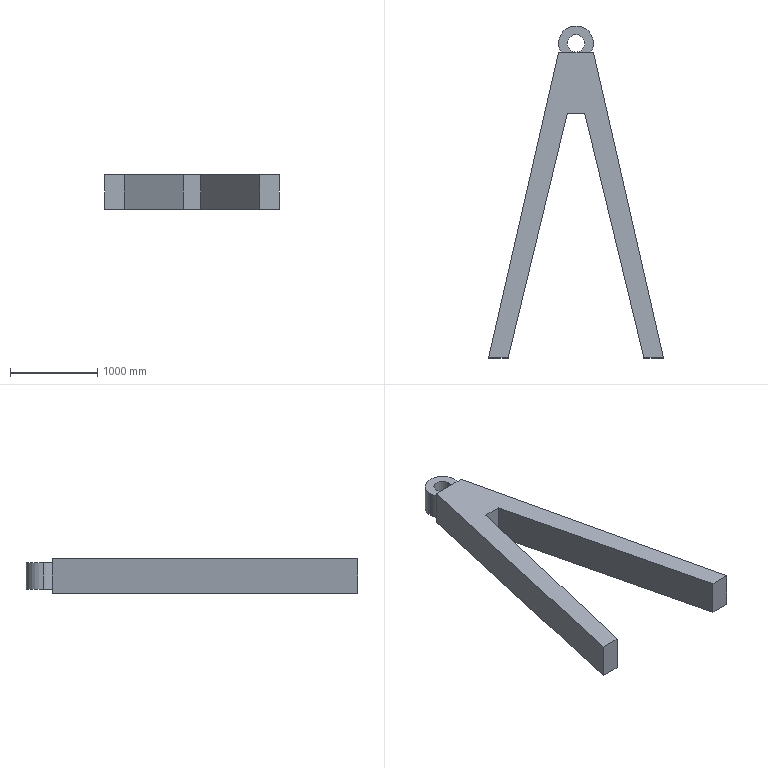Part | SolidWorks | features ICE 2, Extrusion 1 | 1 solid | 17 faces | box 2000 x 3800 x 400 mm | volume 719938598 mm3 | plane 12 | cylinder 5 | commonest cylinder face diameters 400 x3 200 x2
STEP:
#1=CARTESIAN_POINT('',(-100.,0.,-150.));
#2=VERTEX_POINT('',#1);
#3=CARTESIAN_POINT('',(0.,-100.,-150.));
#4=VERTEX_POINT('',#3);
#5=CARTESIAN_POINT('',(0.,0.,-150.));
#6=DIRECTION('',(0.,0.,1.));
#7=DIRECTION('',(1.,0.,0.));
#8=AXIS2_PLACEMENT_3D('',#5,#6,#7);
#9=CIRCLE('',#8,100.);
#10=EDGE_CURVE('',#2,#4,#9,.T.);
#11=ORIENTED_EDGE('',*,*,#10,.F.);
#12=CARTESIAN_POINT('',(-100.,0.,150.));
#13=VERTEX_POINT('',#12);
#14=CARTESIAN_POINT('',(-100.,0.,-150.));
#15=DIRECTION('',(0.,0.,1.));
#16=VECTOR('',#15,1000.);
#17=LINE('',#14,#16);
#18=EDGE_CURVE('',#2,#13,#17,.T.);
#19=ORIENTED_EDGE('',*,*,#18,.T.);
#20=CARTESIAN_POINT('',(0.,-100.,150.));
#21=VERTEX_POINT('',#20);
#22=CARTESIAN_POINT('',(0.,0.,150.));
#23=DIRECTION('',(0.,0.,1.));
#24=DIRECTION('',(1.,0.,0.));
#25=AXIS2_PLACEMENT_3D('',#22,#23,#24);
#26=CIRCLE('',#25,100.);
#27=EDGE_CURVE('',#13,#21,#26,.T.);
#28=ORIENTED_EDGE('',*,*,#27,.T.);
#29=CARTESIAN_POINT('',(100.,0.,150.));
#30=VERTEX_POINT('',#29);
#31=CARTESIAN_POINT('',(0.,0.,150.));
#32=DIRECTION('',(0.,0.,1.));
#33=DIRECTION('',(1.,0.,0.));
#34=AXIS2_PLACEMENT_3D('',#31,#32,#33);
#35=CIRCLE('',#34,100.);
#36=EDGE_CURVE('',#21,#30,#35,.T.);
#37=ORIENTED_EDGE('',*,*,#36,.T.);
#38=CARTESIAN_POINT('',(100.,0.,-150.));
#39=VERTEX_POINT('',#38);
#40=CARTESIAN_POINT('',(100.,0.,-150.));
#41=DIRECTION('',(0.,0.,1.));
#42=VECTOR('',#41,1000.);
#43=LINE('',#40,#42);
#44=EDGE_CURVE('',#39,#30,#43,.T.);
#45=ORIENTED_EDGE('',*,*,#44,.F.);
#46=CARTESIAN_POINT('',(0.,0.,-150.));
#47=DIRECTION('',(0.,0.,1.));
#48=DIRECTION('',(1.,0.,0.));
#49=AXIS2_PLACEMENT_3D('',#46,#47,#48);
#50=CIRCLE('',#49,100.);
#51=EDGE_CURVE('',#4,#39,#50,.T.);
#52=ORIENTED_EDGE('',*,*,#51,.F.);
#53=EDGE_LOOP('',(#11,#19,#28,#37,#45,#52));
#54=FACE_OUTER_BOUND('',#53,.T.);
#55=CARTESIAN_POINT('',(0.,0.,-150.));
#56=DIRECTION('',(0.,0.,1.));
#57=DIRECTION('',(1.,0.,0.));
#58=AXIS2_PLACEMENT_3D('',#55,#56,#57);
#59=CYLINDRICAL_SURFACE('',#58,100.);
#60=ADVANCED_FACE('',(#54),#59,.F.);
#61=CARTESIAN_POINT('',(200.,0.,-150.));
#62=VERTEX_POINT('',#61);
#63=CARTESIAN_POINT('',(-200.,0.,-150.));
#64=VERTEX_POINT('',#63);
#65=CARTESIAN_POINT('',(0.,0.,-150.));
#66=DIRECTION('',(0.,0.,1.));
#67=DIRECTION('',(1.,0.,0.));
#68=AXIS2_PLACEMENT_3D('',#65,#66,#67);
#69=CIRCLE('',#68,200.);
#70=EDGE_CURVE('',#62,#64,#69,.T.);
#71=ORIENTED_EDGE('',*,*,#70,.T.);
#72=CARTESIAN_POINT('',(-200.,0.,150.));
#73=VERTEX_POINT('',#72);
#74=CARTESIAN_POINT('',(-200.,0.,-150.));
#75=DIRECTION('',(0.,0.,1.));
#76=VECTOR('',#75,1000.);
#77=LINE('',#74,#76);
#78=EDGE_CURVE('',#64,#73,#77,.T.);
#79=ORIENTED_EDGE('',*,*,#78,.T.);
#80=CARTESIAN_POINT('',(200.,0.,150.));
#81=VERTEX_POINT('',#80);
#82=CARTESIAN_POINT('',(0.,0.,150.));
#83=DIRECTION('',(0.,0.,1.));
#84=DIRECTION('',(1.,0.,0.));
#85=AXIS2_PLACEMENT_3D('',#82,#83,#84);
#86=CIRCLE('',#85,200.);
#87=EDGE_CURVE('',#81,#73,#86,.T.);
#88=ORIENTED_EDGE('',*,*,#87,.F.);
#89=CARTESIAN_POINT('',(200.,0.,-150.));
#90=DIRECTION('',(0.,0.,1.));
#91=VECTOR('',#90,1000.);
#92=LINE('',#89,#91);
#93=EDGE_CURVE('',#62,#81,#92,.T.);
#94=ORIENTED_EDGE('',*,*,#93,.F.);
#95=EDGE_LOOP('',(#71,#79,#88,#94));
#96=FACE_OUTER_BOUND('',#95,.T.);
#97=CARTESIAN_POINT('',(0.,0.,-150.));
#98=DIRECTION('',(0.,0.,1.));
#99=DIRECTION('',(1.,0.,0.));
#100=AXIS2_PLACEMENT_3D('',#97,#98,#99);
#101=CYLINDRICAL_SURFACE('',#100,200.);
#102=ADVANCED_FACE('',(#96),#101,.T.);
#103=CARTESIAN_POINT('',(173.205,-100.,-150.));
#104=VERTEX_POINT('',#103);
#105=CARTESIAN_POINT('',(0.,0.,-150.));
#106=DIRECTION('',(0.,0.,1.));
#107=DIRECTION('',(1.,0.,0.));
#108=AXIS2_PLACEMENT_3D('',#105,#106,#107);
#109=CIRCLE('',#108,200.);
#110=EDGE_CURVE('',#104,#62,#109,.T.);
#111=ORIENTED_EDGE('',*,*,#110,.T.);
#112=ORIENTED_EDGE('',*,*,#93,.T.);
#113=CARTESIAN_POINT('',(173.205,-100.,150.));
#114=VERTEX_POINT('',#113);
#115=CARTESIAN_POINT('',(0.,0.,150.));
#116=DIRECTION('',(0.,0.,1.));
#117=DIRECTION('',(1.,0.,0.));
#118=AXIS2_PLACEMENT_3D('',#115,#116,#117);
#119=CIRCLE('',#118,200.);
#120=EDGE_CURVE('',#114,#81,#119,.T.);
#121=ORIENTED_EDGE('',*,*,#120,.F.);
#122=CARTESIAN_POINT('',(173.205,-100.,-150.));
#123=DIRECTION('',(0.,0.,1.));
#124=VECTOR('',#123,1000.);
#125=LINE('',#122,#124);
#126=EDGE_CURVE('',#104,#114,#125,.T.);
#127=ORIENTED_EDGE('',*,*,#126,.F.);
#128=EDGE_LOOP('',(#111,#112,#121,#127));
#129=FACE_OUTER_BOUND('',#128,.T.);
#130=CARTESIAN_POINT('',(0.,0.,-150.));
#131=DIRECTION('',(0.,0.,1.));
#132=DIRECTION('',(1.,0.,0.));
#133=AXIS2_PLACEMENT_3D('',#130,#131,#132);
#134=CYLINDRICAL_SURFACE('',#133,200.);
#135=ADVANCED_FACE('',(#129),#134,.T.);
#136=CARTESIAN_POINT('',(-1000.,-3600.,-200.));
#137=VERTEX_POINT('',#136);
#138=CARTESIAN_POINT('',(-775.862,-3600.,-200.));
#139=VERTEX_POINT('',#138);
#140=CARTESIAN_POINT('',(1000.,-3600.,-200.));
#141=DIRECTION('',(1.,0.,0.));
#142=VECTOR('',#141,1000.);
#143=LINE('',#140,#142);
#144=EDGE_CURVE('',#137,#139,#143,.T.);
#145=ORIENTED_EDGE('',*,*,#144,.T.);
#146=CARTESIAN_POINT('',(-775.862,-3600.,200.));
#147=VERTEX_POINT('',#146);
#148=CARTESIAN_POINT('',(-775.862,-3600.,-200.));
#149=DIRECTION('',(0.,0.,1.));
#150=VECTOR('',#149,1000.);
#151=LINE('',#148,#150);
#152=EDGE_CURVE('',#139,#147,#151,.T.);
#153=ORIENTED_EDGE('',*,*,#152,.T.);
#154=CARTESIAN_POINT('',(-1000.,-3600.,200.));
#155=VERTEX_POINT('',#154);
#156=CARTESIAN_POINT('',(1000.,-3600.,200.));
#157=DIRECTION('',(1.,0.,0.));
#158=VECTOR('',#157,1000.);
#159=LINE('',#156,#158);
#160=EDGE_CURVE('',#155,#147,#159,.T.);
#161=ORIENTED_EDGE('',*,*,#160,.F.);
#162=CARTESIAN_POINT('',(-1000.,-3600.,-200.));
#163=DIRECTION('',(0.,0.,1.));
#164=VECTOR('',#163,1000.);
#165=LINE('',#162,#164);
#166=EDGE_CURVE('',#137,#155,#165,.T.);
#167=ORIENTED_EDGE('',*,*,#166,.F.);
#168=EDGE_LOOP('',(#145,#153,#161,#167));
#169=FACE_OUTER_BOUND('',#168,.T.);
#170=CARTESIAN_POINT('',(1000.,-3600.,-200.));
#171=DIRECTION('',(0.,-1.,0.));
#172=DIRECTION('',(1.,0.,0.));
#173=AXIS2_PLACEMENT_3D('',#170,#171,#172);
#174=PLANE('',#173);
#175=ADVANCED_FACE('',(#169),#174,.T.);
#176=CARTESIAN_POINT('',(775.862,-3600.,200.));
#177=VERTEX_POINT('',#176);
#178=CARTESIAN_POINT('',(1000.,-3600.,200.));
#179=VERTEX_POINT('',#178);
#180=CARTESIAN_POINT('',(1000.,-3600.,200.));
#181=DIRECTION('',(1.,0.,0.));
#182=VECTOR('',#181,1000.);
#183=LINE('',#180,#182);
#184=EDGE_CURVE('',#177,#179,#183,.T.);
#185=ORIENTED_EDGE('',*,*,#184,.F.);
#186=CARTESIAN_POINT('',(775.862,-3600.,-200.));
#187=VERTEX_POINT('',#186);
#188=CARTESIAN_POINT('',(775.862,-3600.,-200.));
#189=DIRECTION('',(0.,0.,-1.));
#190=VECTOR('',#189,1000.);
#191=LINE('',#188,#190);
#192=EDGE_CURVE('',#177,#187,#191,.T.);
#193=ORIENTED_EDGE('',*,*,#192,.T.);
#194=CARTESIAN_POINT('',(1000.,-3600.,-200.));
#195=VERTEX_POINT('',#194);
#196=CARTESIAN_POINT('',(1000.,-3600.,-200.));
#197=DIRECTION('',(1.,0.,0.));
#198=VECTOR('',#197,1000.);
#199=LINE('',#196,#198);
#200=EDGE_CURVE('',#187,#195,#199,.T.);
#201=ORIENTED_EDGE('',*,*,#200,.T.);
#202=CARTESIAN_POINT('',(1000.,-3600.,-200.));
#203=DIRECTION('',(0.,0.,1.));
#204=VECTOR('',#203,1000.);
#205=LINE('',#202,#204);
#206=EDGE_CURVE('',#195,#179,#205,.T.);
#207=ORIENTED_EDGE('',*,*,#206,.T.);
#208=EDGE_LOOP('',(#185,#193,#201,#207));
#209=FACE_OUTER_BOUND('',#208,.T.);
#210=CARTESIAN_POINT('',(1000.,-3600.,-200.));
#211=DIRECTION('',(0.,-1.,0.));
#212=DIRECTION('',(1.,0.,0.));
#213=AXIS2_PLACEMENT_3D('',#210,#211,#212);
#214=PLANE('',#213);
#215=ADVANCED_FACE('',(#209),#214,.T.);
#216=CARTESIAN_POINT('',(100.,-800.,-200.));
#217=VERTEX_POINT('',#216);
#218=CARTESIAN_POINT('',(-100.,-800.,-200.));
#219=VERTEX_POINT('',#218);
#220=CARTESIAN_POINT('',(-200.,-800.,-200.));
#221=DIRECTION('',(-1.,0.,0.));
#222=VECTOR('',#221,1000.);
#223=LINE('',#220,#222);
#224=EDGE_CURVE('',#217,#219,#223,.T.);
#225=ORIENTED_EDGE('',*,*,#224,.T.);
#226=CARTESIAN_POINT('',(54.157,-161.348,-200.));
#227=DIRECTION('',(-0.2346,-0.9721,0.));
#228=VECTOR('',#227,1000.);
#229=LINE('',#226,#228);
#230=EDGE_CURVE('',#219,#139,#229,.T.);
#231=ORIENTED_EDGE('',*,*,#230,.T.);
#232=ORIENTED_EDGE('',*,*,#144,.F.);
#233=CARTESIAN_POINT('',(-200.,-100.,-200.));
#234=VERTEX_POINT('',#233);
#235=CARTESIAN_POINT('',(-1000.,-3600.,-200.));
#236=DIRECTION('',(-0.2228,-0.9749,0.));
#237=VECTOR('',#236,1000.);
#238=LINE('',#235,#237);
#239=EDGE_CURVE('',#234,#137,#238,.T.);
#240=ORIENTED_EDGE('',*,*,#239,.F.);
#241=CARTESIAN_POINT('',(200.,-100.,-200.));
#242=VERTEX_POINT('',#241);
#243=CARTESIAN_POINT('',(-200.,-100.,-200.));
#244=DIRECTION('',(-1.,0.,0.));
#245=VECTOR('',#244,1000.);
#246=LINE('',#243,#245);
#247=EDGE_CURVE('',#242,#234,#246,.T.);
#248=ORIENTED_EDGE('',*,*,#247,.F.);
#249=CARTESIAN_POINT('',(200.,-100.,-200.));
#250=DIRECTION('',(-0.2228,0.9749,0.));
#251=VECTOR('',#250,1000.);
#252=LINE('',#249,#251);
#253=EDGE_CURVE('',#195,#242,#252,.T.);
#254=ORIENTED_EDGE('',*,*,#253,.F.);
#255=ORIENTED_EDGE('',*,*,#200,.F.);
#256=CARTESIAN_POINT('',(-76.18,-70.112,-200.));
#257=DIRECTION('',(-0.2346,0.9721,0.));
#258=VECTOR('',#257,1000.);
#259=LINE('',#256,#258);
#260=EDGE_CURVE('',#187,#217,#259,.T.);
#261=ORIENTED_EDGE('',*,*,#260,.T.);
#262=EDGE_LOOP('',(#225,#231,#232,#240,#248,#254,#255,#261));
#263=FACE_OUTER_BOUND('',#262,.T.);
#264=CARTESIAN_POINT('',(-200.,-100.,-200.));
#265=DIRECTION('',(0.,0.,-1.));
#266=DIRECTION('',(-1.,0.,0.));
#267=AXIS2_PLACEMENT_3D('',#264,#265,#266);
#268=PLANE('',#267);
#269=ADVANCED_FACE('',(#263),#268,.T.);
#270=CARTESIAN_POINT('',(-100.,-800.,200.));
#271=VERTEX_POINT('',#270);
#272=CARTESIAN_POINT('',(54.157,-161.348,200.));
#273=DIRECTION('',(-0.2346,-0.9721,0.));
#274=VECTOR('',#273,1000.);
#275=LINE('',#272,#274);
#276=EDGE_CURVE('',#271,#147,#275,.T.);
#277=ORIENTED_EDGE('',*,*,#276,.F.);
#278=CARTESIAN_POINT('',(100.,-800.,200.));
#279=VERTEX_POINT('',#278);
#280=CARTESIAN_POINT('',(-200.,-800.,200.));
#281=DIRECTION('',(-1.,0.,0.));
#282=VECTOR('',#281,1000.);
#283=LINE('',#280,#282);
#284=EDGE_CURVE('',#279,#271,#283,.T.);
#285=ORIENTED_EDGE('',*,*,#284,.F.);
#286=CARTESIAN_POINT('',(-76.18,-70.112,200.));
#287=DIRECTION('',(-0.2346,0.9721,0.));
#288=VECTOR('',#287,1000.);
#289=LINE('',#286,#288);
#290=EDGE_CURVE('',#177,#279,#289,.T.);
#291=ORIENTED_EDGE('',*,*,#290,.F.);
#292=ORIENTED_EDGE('',*,*,#184,.T.);
#293=CARTESIAN_POINT('',(200.,-100.,200.));
#294=VERTEX_POINT('',#293);
#295=CARTESIAN_POINT('',(200.,-100.,200.));
#296=DIRECTION('',(-0.2228,0.9749,0.));
#297=VECTOR('',#296,1000.);
#298=LINE('',#295,#297);
#299=EDGE_CURVE('',#179,#294,#298,.T.);
#300=ORIENTED_EDGE('',*,*,#299,.T.);
#301=CARTESIAN_POINT('',(-200.,-100.,200.));
#302=VERTEX_POINT('',#301);
#303=CARTESIAN_POINT('',(-200.,-100.,200.));
#304=DIRECTION('',(-1.,0.,0.));
#305=VECTOR('',#304,1000.);
#306=LINE('',#303,#305);
#307=EDGE_CURVE('',#294,#302,#306,.T.);
#308=ORIENTED_EDGE('',*,*,#307,.T.);
#309=CARTESIAN_POINT('',(-1000.,-3600.,200.));
#310=DIRECTION('',(-0.2228,-0.9749,0.));
#311=VECTOR('',#310,1000.);
#312=LINE('',#309,#311);
#313=EDGE_CURVE('',#302,#155,#312,.T.);
#314=ORIENTED_EDGE('',*,*,#313,.T.);
#315=ORIENTED_EDGE('',*,*,#160,.T.);
#316=EDGE_LOOP('',(#277,#285,#291,#292,#300,#308,#314,#315));
#317=FACE_OUTER_BOUND('',#316,.T.);
#318=CARTESIAN_POINT('',(-200.,-100.,200.));
#319=DIRECTION('',(0.,0.,-1.));
#320=DIRECTION('',(-1.,0.,0.));
#321=AXIS2_PLACEMENT_3D('',#318,#319,#320);
#322=PLANE('',#321);
#323=ADVANCED_FACE('',(#317),#322,.F.);
#324=ORIENTED_EDGE('',*,*,#78,.F.);
#325=CARTESIAN_POINT('',(-173.205,-100.,-150.));
#326=VERTEX_POINT('',#325);
#327=CARTESIAN_POINT('',(0.,0.,-150.));
#328=DIRECTION('',(0.,0.,1.));
#329=DIRECTION('',(1.,0.,0.));
#330=AXIS2_PLACEMENT_3D('',#327,#328,#329);
#331=CIRCLE('',#330,200.);
#332=EDGE_CURVE('',#64,#326,#331,.T.);
#333=ORIENTED_EDGE('',*,*,#332,.T.);
#334=CARTESIAN_POINT('',(-173.205,-100.,150.));
#335=VERTEX_POINT('',#334);
#336=CARTESIAN_POINT('',(-173.205,-100.,-150.));
#337=DIRECTION('',(0.,0.,-1.));
#338=VECTOR('',#337,1000.);
#339=LINE('',#336,#338);
#340=EDGE_CURVE('',#335,#326,#339,.T.);
#341=ORIENTED_EDGE('',*,*,#340,.F.);
#342=CARTESIAN_POINT('',(0.,0.,150.));
#343=DIRECTION('',(0.,0.,1.));
#344=DIRECTION('',(1.,0.,0.));
#345=AXIS2_PLACEMENT_3D('',#342,#343,#344);
#346=CIRCLE('',#345,200.);
#347=EDGE_CURVE('',#73,#335,#346,.T.);
#348=ORIENTED_EDGE('',*,*,#347,.F.);
#349=EDGE_LOOP('',(#324,#333,#341,#348));
#350=FACE_OUTER_BOUND('',#349,.T.);
#351=CARTESIAN_POINT('',(0.,0.,-150.));
#352=DIRECTION('',(0.,0.,1.));
#353=DIRECTION('',(1.,0.,0.));
#354=AXIS2_PLACEMENT_3D('',#351,#352,#353);
#355=CYLINDRICAL_SURFACE('',#354,200.);
#356=ADVANCED_FACE('',(#350),#355,.T.);
#357=ORIENTED_EDGE('',*,*,#110,.F.);
#358=CARTESIAN_POINT('',(0.,-100.,-150.));
#359=DIRECTION('',(-1.,0.,0.));
#360=VECTOR('',#359,1000.);
#361=LINE('',#358,#360);
#362=EDGE_CURVE('',#104,#4,#361,.T.);
#363=ORIENTED_EDGE('',*,*,#362,.T.);
#364=ORIENTED_EDGE('',*,*,#51,.T.);
#365=CARTESIAN_POINT('',(0.,0.,-150.));
#366=DIRECTION('',(0.,0.,1.));
#367=DIRECTION('',(1.,0.,0.));
#368=AXIS2_PLACEMENT_3D('',#365,#366,#367);
#369=CIRCLE('',#368,100.);
#370=EDGE_CURVE('',#39,#2,#369,.T.);
#371=ORIENTED_EDGE('',*,*,#370,.T.);
#372=ORIENTED_EDGE('',*,*,#10,.T.);
#373=CARTESIAN_POINT('',(0.,-100.,-150.));
#374=DIRECTION('',(-1.,0.,0.));
#375=VECTOR('',#374,1000.);
#376=LINE('',#373,#375);
#377=EDGE_CURVE('',#4,#326,#376,.T.);
#378=ORIENTED_EDGE('',*,*,#377,.T.);
#379=ORIENTED_EDGE('',*,*,#332,.F.);
#380=ORIENTED_EDGE('',*,*,#70,.F.);
#381=EDGE_LOOP('',(#357,#363,#364,#371,#372,#378,#379,#380));
#382=FACE_OUTER_BOUND('',#381,.T.);
#383=CARTESIAN_POINT('',(0.,0.,-150.));
#384=DIRECTION('',(0.,0.,1.));
#385=DIRECTION('',(1.,0.,0.));
#386=AXIS2_PLACEMENT_3D('',#383,#384,#385);
#387=PLANE('',#386);
#388=ADVANCED_FACE('',(#382),#387,.F.);
#389=ORIENTED_EDGE('',*,*,#18,.F.);
#390=ORIENTED_EDGE('',*,*,#370,.F.);
#391=ORIENTED_EDGE('',*,*,#44,.T.);
#392=CARTESIAN_POINT('',(0.,0.,150.));
#393=DIRECTION('',(0.,0.,1.));
#394=DIRECTION('',(1.,0.,0.));
#395=AXIS2_PLACEMENT_3D('',#392,#393,#394);
#396=CIRCLE('',#395,100.);
#397=EDGE_CURVE('',#30,#13,#396,.T.);
#398=ORIENTED_EDGE('',*,*,#397,.T.);
#399=EDGE_LOOP('',(#389,#390,#391,#398));
#400=FACE_OUTER_BOUND('',#399,.T.);
#401=CARTESIAN_POINT('',(0.,0.,-150.));
#402=DIRECTION('',(0.,0.,1.));
#403=DIRECTION('',(1.,0.,0.));
#404=AXIS2_PLACEMENT_3D('',#401,#402,#403);
#405=CYLINDRICAL_SURFACE('',#404,100.);
#406=ADVANCED_FACE('',(#400),#405,.F.);
#407=CARTESIAN_POINT('',(0.,-100.,150.));
#408=DIRECTION('',(-1.,0.,0.));
#409=VECTOR('',#408,1000.);
#410=LINE('',#407,#409);
#411=EDGE_CURVE('',#114,#21,#410,.T.);
#412=ORIENTED_EDGE('',*,*,#411,.F.);
#413=ORIENTED_EDGE('',*,*,#120,.T.);
#414=ORIENTED_EDGE('',*,*,#87,.T.);
#415=ORIENTED_EDGE('',*,*,#347,.T.);
#416=CARTESIAN_POINT('',(0.,-100.,150.));
#417=DIRECTION('',(-1.,0.,0.));
#418=VECTOR('',#417,1000.);
#419=LINE('',#416,#418);
#420=EDGE_CURVE('',#21,#335,#419,.T.);
#421=ORIENTED_EDGE('',*,*,#420,.F.);
#422=ORIENTED_EDGE('',*,*,#27,.F.);
#423=ORIENTED_EDGE('',*,*,#397,.F.);
#424=ORIENTED_EDGE('',*,*,#36,.F.);
#425=EDGE_LOOP('',(#412,#413,#414,#415,#421,#422,#423,#424));
#426=FACE_OUTER_BOUND('',#425,.T.);
#427=CARTESIAN_POINT('',(0.,0.,150.));
#428=DIRECTION('',(0.,0.,1.));
#429=DIRECTION('',(1.,0.,0.));
#430=AXIS2_PLACEMENT_3D('',#427,#428,#429);
#431=PLANE('',#430);
#432=ADVANCED_FACE('',(#426),#431,.T.);
#433=CARTESIAN_POINT('',(-200.,-100.,-200.));
#434=DIRECTION('',(0.,0.,1.));
#435=VECTOR('',#434,1000.);
#436=LINE('',#433,#435);
#437=EDGE_CURVE('',#234,#302,#436,.T.);
#438=ORIENTED_EDGE('',*,*,#437,.T.);
#439=ORIENTED_EDGE('',*,*,#307,.F.);
#440=CARTESIAN_POINT('',(200.,-100.,-200.));
#441=DIRECTION('',(0.,0.,1.));
#442=VECTOR('',#441,1000.);
#443=LINE('',#440,#442);
#444=EDGE_CURVE('',#242,#294,#443,.T.);
#445=ORIENTED_EDGE('',*,*,#444,.F.);
#446=ORIENTED_EDGE('',*,*,#247,.T.);
#447=EDGE_LOOP('',(#438,#439,#445,#446));
#448=FACE_OUTER_BOUND('',#447,.T.);
#449=ORIENTED_EDGE('',*,*,#362,.F.);
#450=ORIENTED_EDGE('',*,*,#126,.T.);
#451=ORIENTED_EDGE('',*,*,#411,.T.);
#452=ORIENTED_EDGE('',*,*,#420,.T.);
#453=ORIENTED_EDGE('',*,*,#340,.T.);
#454=ORIENTED_EDGE('',*,*,#377,.F.);
#455=EDGE_LOOP('',(#449,#450,#451,#452,#453,#454));
#456=FACE_BOUND('',#455,.T.);
#457=CARTESIAN_POINT('',(-200.,-100.,-200.));
#458=DIRECTION('',(0.,1.,0.));
#459=DIRECTION('',(0.,0.,1.));
#460=AXIS2_PLACEMENT_3D('',#457,#458,#459);
#461=PLANE('',#460);
#462=ADVANCED_FACE('',(#448,#456),#461,.T.);
#463=ORIENTED_EDGE('',*,*,#166,.T.);
#464=ORIENTED_EDGE('',*,*,#313,.F.);
#465=ORIENTED_EDGE('',*,*,#437,.F.);
#466=ORIENTED_EDGE('',*,*,#239,.T.);
#467=EDGE_LOOP('',(#463,#464,#465,#466));
#468=FACE_OUTER_BOUND('',#467,.T.);
#469=CARTESIAN_POINT('',(-1000.,-3600.,-200.));
#470=DIRECTION('',(-0.9749,0.2228,0.));
#471=DIRECTION('',(-0.2228,-0.9749,0.));
#472=AXIS2_PLACEMENT_3D('',#469,#470,#471);
#473=PLANE('',#472);
#474=ADVANCED_FACE('',(#468),#473,.T.);
#475=ORIENTED_EDGE('',*,*,#444,.T.);
#476=ORIENTED_EDGE('',*,*,#299,.F.);
#477=ORIENTED_EDGE('',*,*,#206,.F.);
#478=ORIENTED_EDGE('',*,*,#253,.T.);
#479=EDGE_LOOP('',(#475,#476,#477,#478));
#480=FACE_OUTER_BOUND('',#479,.T.);
#481=CARTESIAN_POINT('',(200.,-100.,-200.));
#482=DIRECTION('',(0.9749,0.2228,0.));
#483=DIRECTION('',(-0.2228,0.9749,0.));
#484=AXIS2_PLACEMENT_3D('',#481,#482,#483);
#485=PLANE('',#484);
#486=ADVANCED_FACE('',(#480),#485,.T.);
#487=CARTESIAN_POINT('',(100.,-800.,700.));
#488=DIRECTION('',(0.,0.,-1.));
#489=VECTOR('',#488,1000.);
#490=LINE('',#487,#489);
#491=EDGE_CURVE('',#279,#217,#490,.T.);
#492=ORIENTED_EDGE('',*,*,#491,.F.);
#493=ORIENTED_EDGE('',*,*,#284,.T.);
#494=CARTESIAN_POINT('',(-100.,-800.,700.));
#495=DIRECTION('',(0.,0.,-1.));
#496=VECTOR('',#495,1000.);
#497=LINE('',#494,#496);
#498=EDGE_CURVE('',#271,#219,#497,.T.);
#499=ORIENTED_EDGE('',*,*,#498,.T.);
#500=ORIENTED_EDGE('',*,*,#224,.F.);
#501=EDGE_LOOP('',(#492,#493,#499,#500));
#502=FACE_OUTER_BOUND('',#501,.T.);
#503=CARTESIAN_POINT('',(-100.,-800.,700.));
#504=DIRECTION('',(0.,-1.,0.));
#505=DIRECTION('',(1.,0.,0.));
#506=AXIS2_PLACEMENT_3D('',#503,#504,#505);
#507=PLANE('',#506);
#508=ADVANCED_FACE('',(#502),#507,.T.);
#509=ORIENTED_EDGE('',*,*,#498,.F.);
#510=ORIENTED_EDGE('',*,*,#276,.T.);
#511=ORIENTED_EDGE('',*,*,#152,.F.);
#512=ORIENTED_EDGE('',*,*,#230,.F.);
#513=EDGE_LOOP('',(#509,#510,#511,#512));
#514=FACE_OUTER_BOUND('',#513,.T.);
#515=CARTESIAN_POINT('',(-800.,-3700.,700.));
#516=DIRECTION('',(0.9721,-0.2346,0.));
#517=DIRECTION('',(0.2346,0.9721,0.));
#518=AXIS2_PLACEMENT_3D('',#515,#516,#517);
#519=PLANE('',#518);
#520=ADVANCED_FACE('',(#514),#519,.T.);
#521=ORIENTED_EDGE('',*,*,#192,.F.);
#522=ORIENTED_EDGE('',*,*,#290,.T.);
#523=ORIENTED_EDGE('',*,*,#491,.T.);
#524=ORIENTED_EDGE('',*,*,#260,.F.);
#525=EDGE_LOOP('',(#521,#522,#523,#524));
#526=FACE_OUTER_BOUND('',#525,.T.);
#527=CARTESIAN_POINT('',(100.,-800.,700.));
#528=DIRECTION('',(-0.9721,-0.2346,0.));
#529=DIRECTION('',(0.2346,-0.9721,0.));
#530=AXIS2_PLACEMENT_3D('',#527,#528,#529);
#531=PLANE('',#530);
#532=ADVANCED_FACE('',(#526),#531,.T.);
#533=CLOSED_SHELL('',(#60,#102,#135,#175,#215,#269,#323,#356,#388,#406,#432,#462,#474,#486,#508,#520,#532));
#534=MANIFOLD_SOLID_BREP('',#533);
#535=CARTESIAN_POINT('',(0.,0.,0.));
#536=DIRECTION('',(0.,0.,1.));
#537=DIRECTION('',(1.,0.,0.));
#538=AXIS2_PLACEMENT_3D('',#535,#536,#537);
#539=(LENGTH_UNIT()NAMED_UNIT(*)SI_UNIT(.MILLI.,.METRE.));
#540=UNCERTAINTY_MEASURE_WITH_UNIT(LENGTH_MEASURE(0.00001),#539,'','');
#541=(NAMED_UNIT(*)PLANE_ANGLE_UNIT()SI_UNIT($,.RADIAN.));
#542=(NAMED_UNIT(*)SI_UNIT($,.STERADIAN.)SOLID_ANGLE_UNIT());
#543=(GEOMETRIC_REPRESENTATION_CONTEXT(3)GLOBAL_UNCERTAINTY_ASSIGNED_CONTEXT((#540))GLOBAL_UNIT_ASSIGNED_CONTEXT((#539,#541,#542))REPRESENTATION_CONTEXT('',''));
#544=ADVANCED_BREP_SHAPE_REPRESENTATION('',(#534,#538),#543);